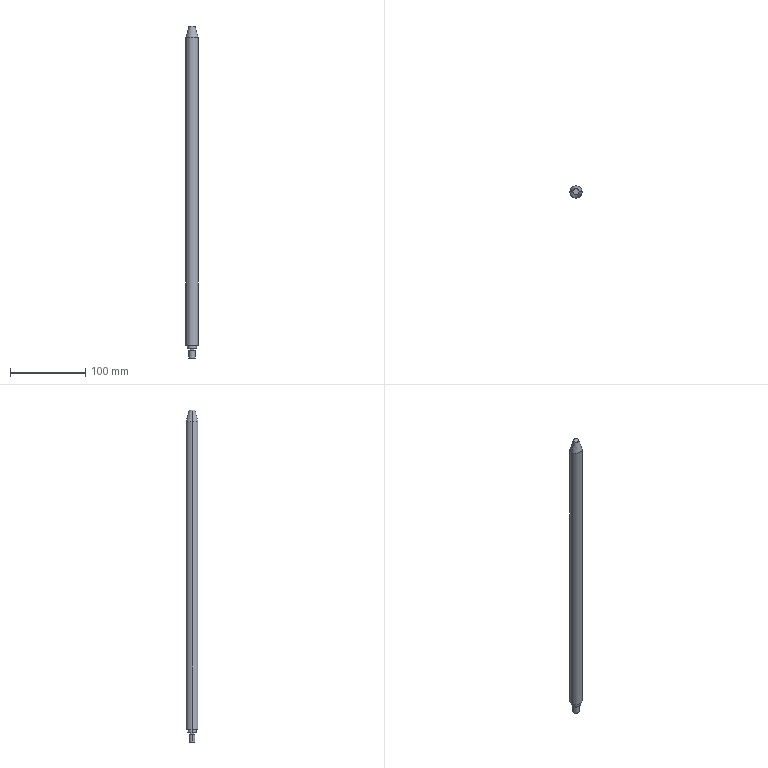Part | STEP file | Stop rod_default<machined> | 1 solid | 15 faces | box 16 x 16 x 440 mm | volume 84922 mm3 | cylinder 8 | plane 5 | cone 2 | commonest cylinder face diameters 6.5 x2 8 x2 12 x2 16 x2
STEP:
#1=CARTESIAN_POINT('',(0.,0.,0.));
#2=DIRECTION('',(0.,0.,1.));
#3=DIRECTION('',(1.,0.,0.));
#4=AXIS2_PLACEMENT_3D('',#1,#2,#3);
#5=CARTESIAN_POINT('',(6.,0.,12.));
#6=VERTEX_POINT('',#5);
#7=CARTESIAN_POINT('',(-6.,0.,12.));
#8=VERTEX_POINT('',#7);
#9=CARTESIAN_POINT('',(0.,0.,12.));
#10=DIRECTION('',(0.,0.,1.));
#11=DIRECTION('',(1.,0.,0.));
#12=AXIS2_PLACEMENT_3D('',#9,#10,#11);
#13=CIRCLE('',#12,6.);
#14=CARTESIAN_POINT('',(0.,0.,1000.));
#15=DIRECTION('',(0.,0.,1.));
#16=DIRECTION('',(1.,0.,0.));
#17=AXIS2_PLACEMENT_3D('',#14,#15,#16);
#18=CYLINDRICAL_SURFACE('',#17,6.);
#19=CARTESIAN_POINT('',(0.,-988.));
#20=DIRECTION('',(1.,0.));
#21=VECTOR('',#20,1.);
#22=LINE('',#19,#21);
#23=(GEOMETRIC_REPRESENTATION_CONTEXT(2)PARAMETRIC_REPRESENTATION_CONTEXT()REPRESENTATION_CONTEXT('',''));
#24=DEFINITIONAL_REPRESENTATION('',(#22),#23);
#25=PCURVE('',#18,#24);
#26=CARTESIAN_POINT('',(3.25,0.,12.));
#27=DIRECTION('',(0.,0.,1.));
#28=DIRECTION('',(1.,0.,0.));
#29=AXIS2_PLACEMENT_3D('',#26,#27,#28);
#30=PLANE('',#29);
#31=CARTESIAN_POINT('',(-3.25,0.));
#32=DIRECTION('',(1.,0.));
#33=AXIS2_PLACEMENT_2D('',#31,#32);
#34=CIRCLE('',#33,6.);
#35=(GEOMETRIC_REPRESENTATION_CONTEXT(2)PARAMETRIC_REPRESENTATION_CONTEXT()REPRESENTATION_CONTEXT('',''));
#36=DEFINITIONAL_REPRESENTATION('',(#34),#35);
#37=PCURVE('',#30,#36);
#38=SURFACE_CURVE('',#13,(#25,#37),.PCURVE_S1.);
#39=EDGE_CURVE('',#6,#8,#38,.T.);
#40=ORIENTED_EDGE('',*,*,#39,.T.);
#41=CARTESIAN_POINT('',(-6.,0.,17.));
#42=VERTEX_POINT('',#41);
#43=CARTESIAN_POINT('',(-6.,0.,1000.));
#44=DIRECTION('',(0.,0.,1.));
#45=VECTOR('',#44,1.);
#46=LINE('',#43,#45);
#47=CARTESIAN_POINT('',(3.142,0.));
#48=DIRECTION('',(0.,1.));
#49=VECTOR('',#48,1.);
#50=LINE('',#47,#49);
#51=(GEOMETRIC_REPRESENTATION_CONTEXT(2)PARAMETRIC_REPRESENTATION_CONTEXT()REPRESENTATION_CONTEXT('',''));
#52=DEFINITIONAL_REPRESENTATION('',(#50),#51);
#53=PCURVE('',#18,#52);
#54=CARTESIAN_POINT('',(0.,0.,1000.));
#55=DIRECTION('',(0.,0.,1.));
#56=DIRECTION('',(1.,0.,0.));
#57=AXIS2_PLACEMENT_3D('',#54,#55,#56);
#58=CYLINDRICAL_SURFACE('',#57,6.);
#59=CARTESIAN_POINT('',(3.142,0.));
#60=DIRECTION('',(0.,1.));
#61=VECTOR('',#60,1.);
#62=LINE('',#59,#61);
#63=(GEOMETRIC_REPRESENTATION_CONTEXT(2)PARAMETRIC_REPRESENTATION_CONTEXT()REPRESENTATION_CONTEXT('',''));
#64=DEFINITIONAL_REPRESENTATION('',(#62),#63);
#65=PCURVE('',#58,#64);
#66=SURFACE_CURVE('',#46,(#53,#65),.PCURVE_S1.);
#67=EDGE_CURVE('',#8,#42,#66,.T.);
#68=ORIENTED_EDGE('',*,*,#67,.T.);
#69=CARTESIAN_POINT('',(6.,0.,17.));
#70=VERTEX_POINT('',#69);
#71=CARTESIAN_POINT('',(0.,0.,17.));
#72=DIRECTION('',(0.,0.,1.));
#73=DIRECTION('',(1.,0.,0.));
#74=AXIS2_PLACEMENT_3D('',#71,#72,#73);
#75=CIRCLE('',#74,6.);
#76=CARTESIAN_POINT('',(0.,-983.));
#77=DIRECTION('',(1.,0.));
#78=VECTOR('',#77,1.);
#79=LINE('',#76,#78);
#80=(GEOMETRIC_REPRESENTATION_CONTEXT(2)PARAMETRIC_REPRESENTATION_CONTEXT()REPRESENTATION_CONTEXT('',''));
#81=DEFINITIONAL_REPRESENTATION('',(#79),#80);
#82=PCURVE('',#18,#81);
#83=CARTESIAN_POINT('',(6.,0.,17.));
#84=DIRECTION('',(0.,0.,1.));
#85=DIRECTION('',(1.,0.,0.));
#86=AXIS2_PLACEMENT_3D('',#83,#84,#85);
#87=PLANE('',#86);
#88=CARTESIAN_POINT('',(-6.,0.));
#89=DIRECTION('',(1.,0.));
#90=AXIS2_PLACEMENT_2D('',#88,#89);
#91=CIRCLE('',#90,6.);
#92=(GEOMETRIC_REPRESENTATION_CONTEXT(2)PARAMETRIC_REPRESENTATION_CONTEXT()REPRESENTATION_CONTEXT('',''));
#93=DEFINITIONAL_REPRESENTATION('',(#91),#92);
#94=PCURVE('',#87,#93);
#95=SURFACE_CURVE('',#75,(#82,#94),.PCURVE_S1.);
#96=EDGE_CURVE('',#70,#42,#95,.T.);
#97=ORIENTED_EDGE('',*,*,#96,.F.);
#98=CARTESIAN_POINT('',(6.,0.,1000.));
#99=DIRECTION('',(0.,0.,1.));
#100=VECTOR('',#99,1.);
#101=LINE('',#98,#100);
#102=CARTESIAN_POINT('',(0.,0.));
#103=DIRECTION('',(0.,1.));
#104=VECTOR('',#103,1.);
#105=LINE('',#102,#104);
#106=(GEOMETRIC_REPRESENTATION_CONTEXT(2)PARAMETRIC_REPRESENTATION_CONTEXT()REPRESENTATION_CONTEXT('',''));
#107=DEFINITIONAL_REPRESENTATION('',(#105),#106);
#108=PCURVE('',#18,#107);
#109=CARTESIAN_POINT('',(6.283,0.));
#110=DIRECTION('',(0.,1.));
#111=VECTOR('',#110,1.);
#112=LINE('',#109,#111);
#113=(GEOMETRIC_REPRESENTATION_CONTEXT(2)PARAMETRIC_REPRESENTATION_CONTEXT()REPRESENTATION_CONTEXT('',''));
#114=DEFINITIONAL_REPRESENTATION('',(#112),#113);
#115=PCURVE('',#58,#114);
#116=SURFACE_CURVE('',#101,(#108,#115),.PCURVE_S1.);
#117=EDGE_CURVE('',#6,#70,#116,.T.);
#118=ORIENTED_EDGE('',*,*,#117,.F.);
#119=EDGE_LOOP('',(#40,#68,#97,#118));
#120=FACE_BOUND('',#119,.T.);
#121=ADVANCED_FACE('',(#120),#18,.T.);
#122=CARTESIAN_POINT('',(3.25,0.,10.));
#123=VERTEX_POINT('',#122);
#124=CARTESIAN_POINT('',(-3.25,0.,10.));
#125=VERTEX_POINT('',#124);
#126=CARTESIAN_POINT('',(0.,0.,10.));
#127=DIRECTION('',(0.,0.,1.));
#128=DIRECTION('',(1.,0.,0.));
#129=AXIS2_PLACEMENT_3D('',#126,#127,#128);
#130=CIRCLE('',#129,3.25);
#131=CARTESIAN_POINT('',(0.,0.,1000.));
#132=DIRECTION('',(0.,0.,1.));
#133=DIRECTION('',(1.,0.,0.));
#134=AXIS2_PLACEMENT_3D('',#131,#132,#133);
#135=CYLINDRICAL_SURFACE('',#134,3.25);
#136=CARTESIAN_POINT('',(0.,-990.));
#137=DIRECTION('',(1.,0.));
#138=VECTOR('',#137,1.);
#139=LINE('',#136,#138);
#140=(GEOMETRIC_REPRESENTATION_CONTEXT(2)PARAMETRIC_REPRESENTATION_CONTEXT()REPRESENTATION_CONTEXT('',''));
#141=DEFINITIONAL_REPRESENTATION('',(#139),#140);
#142=PCURVE('',#135,#141);
#143=CARTESIAN_POINT('',(4.,0.,10.));
#144=DIRECTION('',(0.,0.,-1.));
#145=DIRECTION('',(-1.,0.,0.));
#146=AXIS2_PLACEMENT_3D('',#143,#144,#145);
#147=PLANE('',#146);
#148=CARTESIAN_POINT('',(0.75,0.));
#149=CARTESIAN_POINT('',(0.75,5.629));
#150=CARTESIAN_POINT('',(5.625,2.815));
#151=CARTESIAN_POINT('',(10.5,0.));
#152=CARTESIAN_POINT('',(5.625,-2.815));
#153=CARTESIAN_POINT('',(0.75,-5.629));
#154=CARTESIAN_POINT('',(0.75,0.));
#155=(BOUNDED_CURVE()B_SPLINE_CURVE(2,(#148,#149,#150,#151,#152,#153,#154),.UNSPECIFIED.,.T.,.F.)B_SPLINE_CURVE_WITH_KNOTS((1,2,2,2,2,1),(-2.094,0.,2.094,4.189,6.283,8.378),.UNSPECIFIED.)CURVE()GEOMETRIC_REPRESENTATION_ITEM()RATIONAL_B_SPLINE_CURVE((1.,0.5,1.,0.5,1.,0.5,1.))REPRESENTATION_ITEM(''));
#156=(GEOMETRIC_REPRESENTATION_CONTEXT(2)PARAMETRIC_REPRESENTATION_CONTEXT()REPRESENTATION_CONTEXT('',''));
#157=DEFINITIONAL_REPRESENTATION('',(#155),#156);
#158=PCURVE('',#147,#157);
#159=SURFACE_CURVE('',#130,(#142,#158),.PCURVE_S1.);
#160=EDGE_CURVE('',#123,#125,#159,.T.);
#161=ORIENTED_EDGE('',*,*,#160,.T.);
#162=CARTESIAN_POINT('',(-3.25,0.,12.));
#163=VERTEX_POINT('',#162);
#164=CARTESIAN_POINT('',(-3.25,0.,1000.));
#165=DIRECTION('',(0.,0.,1.));
#166=VECTOR('',#165,1.);
#167=LINE('',#164,#166);
#168=CARTESIAN_POINT('',(3.142,0.));
#169=DIRECTION('',(0.,1.));
#170=VECTOR('',#169,1.);
#171=LINE('',#168,#170);
#172=(GEOMETRIC_REPRESENTATION_CONTEXT(2)PARAMETRIC_REPRESENTATION_CONTEXT()REPRESENTATION_CONTEXT('',''));
#173=DEFINITIONAL_REPRESENTATION('',(#171),#172);
#174=PCURVE('',#135,#173);
#175=CARTESIAN_POINT('',(0.,0.,1000.));
#176=DIRECTION('',(0.,0.,1.));
#177=DIRECTION('',(1.,0.,0.));
#178=AXIS2_PLACEMENT_3D('',#175,#176,#177);
#179=CYLINDRICAL_SURFACE('',#178,3.25);
#180=CARTESIAN_POINT('',(3.142,0.));
#181=DIRECTION('',(0.,1.));
#182=VECTOR('',#181,1.);
#183=LINE('',#180,#182);
#184=(GEOMETRIC_REPRESENTATION_CONTEXT(2)PARAMETRIC_REPRESENTATION_CONTEXT()REPRESENTATION_CONTEXT('',''));
#185=DEFINITIONAL_REPRESENTATION('',(#183),#184);
#186=PCURVE('',#179,#185);
#187=SURFACE_CURVE('',#167,(#174,#186),.PCURVE_S1.);
#188=EDGE_CURVE('',#125,#163,#187,.T.);
#189=ORIENTED_EDGE('',*,*,#188,.T.);
#190=CARTESIAN_POINT('',(3.25,0.,12.));
#191=VERTEX_POINT('',#190);
#192=CARTESIAN_POINT('',(0.,0.,12.));
#193=DIRECTION('',(0.,0.,1.));
#194=DIRECTION('',(1.,0.,0.));
#195=AXIS2_PLACEMENT_3D('',#192,#193,#194);
#196=CIRCLE('',#195,3.25);
#197=CARTESIAN_POINT('',(0.,-988.));
#198=DIRECTION('',(1.,0.));
#199=VECTOR('',#198,1.);
#200=LINE('',#197,#199);
#201=(GEOMETRIC_REPRESENTATION_CONTEXT(2)PARAMETRIC_REPRESENTATION_CONTEXT()REPRESENTATION_CONTEXT('',''));
#202=DEFINITIONAL_REPRESENTATION('',(#200),#201);
#203=PCURVE('',#135,#202);
#204=CARTESIAN_POINT('',(-3.25,0.));
#205=DIRECTION('',(1.,0.));
#206=AXIS2_PLACEMENT_2D('',#204,#205);
#207=CIRCLE('',#206,3.25);
#208=(GEOMETRIC_REPRESENTATION_CONTEXT(2)PARAMETRIC_REPRESENTATION_CONTEXT()REPRESENTATION_CONTEXT('',''));
#209=DEFINITIONAL_REPRESENTATION('',(#207),#208);
#210=PCURVE('',#30,#209);
#211=SURFACE_CURVE('',#196,(#203,#210),.PCURVE_S1.);
#212=EDGE_CURVE('',#191,#163,#211,.T.);
#213=ORIENTED_EDGE('',*,*,#212,.F.);
#214=CARTESIAN_POINT('',(3.25,0.,1000.));
#215=DIRECTION('',(0.,0.,1.));
#216=VECTOR('',#215,1.);
#217=LINE('',#214,#216);
#218=CARTESIAN_POINT('',(0.,0.));
#219=DIRECTION('',(0.,1.));
#220=VECTOR('',#219,1.);
#221=LINE('',#218,#220);
#222=(GEOMETRIC_REPRESENTATION_CONTEXT(2)PARAMETRIC_REPRESENTATION_CONTEXT()REPRESENTATION_CONTEXT('',''));
#223=DEFINITIONAL_REPRESENTATION('',(#221),#222);
#224=PCURVE('',#135,#223);
#225=CARTESIAN_POINT('',(6.283,0.));
#226=DIRECTION('',(0.,1.));
#227=VECTOR('',#226,1.);
#228=LINE('',#225,#227);
#229=(GEOMETRIC_REPRESENTATION_CONTEXT(2)PARAMETRIC_REPRESENTATION_CONTEXT()REPRESENTATION_CONTEXT('',''));
#230=DEFINITIONAL_REPRESENTATION('',(#228),#229);
#231=PCURVE('',#179,#230);
#232=SURFACE_CURVE('',#217,(#224,#231),.PCURVE_S1.);
#233=EDGE_CURVE('',#123,#191,#232,.T.);
#234=ORIENTED_EDGE('',*,*,#233,.F.);
#235=EDGE_LOOP('',(#161,#189,#213,#234));
#236=FACE_BOUND('',#235,.T.);
#237=ADVANCED_FACE('',(#236),#135,.T.);
#238=CARTESIAN_POINT('',(4.,0.,0.));
#239=VERTEX_POINT('',#238);
#240=CARTESIAN_POINT('',(-4.,0.,0.));
#241=VERTEX_POINT('',#240);
#242=CARTESIAN_POINT('',(0.,0.,0.));
#243=DIRECTION('',(0.,0.,1.));
#244=DIRECTION('',(1.,0.,0.));
#245=AXIS2_PLACEMENT_3D('',#242,#243,#244);
#246=CIRCLE('',#245,4.);
#247=CARTESIAN_POINT('',(0.,0.,1000.));
#248=DIRECTION('',(0.,0.,1.));
#249=DIRECTION('',(1.,0.,0.));
#250=AXIS2_PLACEMENT_3D('',#247,#248,#249);
#251=CYLINDRICAL_SURFACE('',#250,4.);
#252=CARTESIAN_POINT('',(0.,-1000.));
#253=DIRECTION('',(1.,0.));
#254=VECTOR('',#253,1.);
#255=LINE('',#252,#254);
#256=(GEOMETRIC_REPRESENTATION_CONTEXT(2)PARAMETRIC_REPRESENTATION_CONTEXT()REPRESENTATION_CONTEXT('',''));
#257=DEFINITIONAL_REPRESENTATION('',(#255),#256);
#258=PCURVE('',#251,#257);
#259=CARTESIAN_POINT('',(0.,0.,0.));
#260=DIRECTION('',(0.,0.,1.));
#261=DIRECTION('',(1.,0.,0.));
#262=AXIS2_PLACEMENT_3D('',#259,#260,#261);
#263=PLANE('',#262);
#264=CARTESIAN_POINT('',(0.,0.));
#265=DIRECTION('',(1.,0.));
#266=AXIS2_PLACEMENT_2D('',#264,#265);
#267=CIRCLE('',#266,4.);
#268=(GEOMETRIC_REPRESENTATION_CONTEXT(2)PARAMETRIC_REPRESENTATION_CONTEXT()REPRESENTATION_CONTEXT('',''));
#269=DEFINITIONAL_REPRESENTATION('',(#267),#268);
#270=PCURVE('',#263,#269);
#271=SURFACE_CURVE('',#246,(#258,#270),.PCURVE_S1.);
#272=EDGE_CURVE('',#239,#241,#271,.T.);
#273=ORIENTED_EDGE('',*,*,#272,.T.);
#274=CARTESIAN_POINT('',(-4.,0.,10.));
#275=VERTEX_POINT('',#274);
#276=CARTESIAN_POINT('',(-4.,0.,1000.));
#277=DIRECTION('',(0.,0.,1.));
#278=VECTOR('',#277,1.);
#279=LINE('',#276,#278);
#280=CARTESIAN_POINT('',(3.142,0.));
#281=DIRECTION('',(0.,1.));
#282=VECTOR('',#281,1.);
#283=LINE('',#280,#282);
#284=(GEOMETRIC_REPRESENTATION_CONTEXT(2)PARAMETRIC_REPRESENTATION_CONTEXT()REPRESENTATION_CONTEXT('',''));
#285=DEFINITIONAL_REPRESENTATION('',(#283),#284);
#286=PCURVE('',#251,#285);
#287=CARTESIAN_POINT('',(0.,0.,1000.));
#288=DIRECTION('',(0.,0.,1.));
#289=DIRECTION('',(1.,0.,0.));
#290=AXIS2_PLACEMENT_3D('',#287,#288,#289);
#291=CYLINDRICAL_SURFACE('',#290,4.);
#292=CARTESIAN_POINT('',(3.142,0.));
#293=DIRECTION('',(0.,1.));
#294=VECTOR('',#293,1.);
#295=LINE('',#292,#294);
#296=(GEOMETRIC_REPRESENTATION_CONTEXT(2)PARAMETRIC_REPRESENTATION_CONTEXT()REPRESENTATION_CONTEXT('',''));
#297=DEFINITIONAL_REPRESENTATION('',(#295),#296);
#298=PCURVE('',#291,#297);
#299=SURFACE_CURVE('',#279,(#286,#298),.PCURVE_S1.);
#300=EDGE_CURVE('',#241,#275,#299,.T.);
#301=ORIENTED_EDGE('',*,*,#300,.T.);
#302=CARTESIAN_POINT('',(4.,0.,10.));
#303=VERTEX_POINT('',#302);
#304=CARTESIAN_POINT('',(0.,0.,10.));
#305=DIRECTION('',(0.,0.,1.));
#306=DIRECTION('',(1.,0.,0.));
#307=AXIS2_PLACEMENT_3D('',#304,#305,#306);
#308=CIRCLE('',#307,4.);
#309=CARTESIAN_POINT('',(0.,-990.));
#310=DIRECTION('',(1.,0.));
#311=VECTOR('',#310,1.);
#312=LINE('',#309,#311);
#313=(GEOMETRIC_REPRESENTATION_CONTEXT(2)PARAMETRIC_REPRESENTATION_CONTEXT()REPRESENTATION_CONTEXT('',''));
#314=DEFINITIONAL_REPRESENTATION('',(#312),#313);
#315=PCURVE('',#251,#314);
#316=CARTESIAN_POINT('',(0.,0.));
#317=CARTESIAN_POINT('',(0.,6.928));
#318=CARTESIAN_POINT('',(6.,3.464));
#319=CARTESIAN_POINT('',(12.,0.));
#320=CARTESIAN_POINT('',(6.,-3.464));
#321=CARTESIAN_POINT('',(0.,-6.928));
#322=CARTESIAN_POINT('',(0.,0.));
#323=(BOUNDED_CURVE()B_SPLINE_CURVE(2,(#316,#317,#318,#319,#320,#321,#322),.UNSPECIFIED.,.T.,.F.)B_SPLINE_CURVE_WITH_KNOTS((1,2,2,2,2,1),(-2.094,0.,2.094,4.189,6.283,8.378),.UNSPECIFIED.)CURVE()GEOMETRIC_REPRESENTATION_ITEM()RATIONAL_B_SPLINE_CURVE((1.,0.5,1.,0.5,1.,0.5,1.))REPRESENTATION_ITEM(''));
#324=(GEOMETRIC_REPRESENTATION_CONTEXT(2)PARAMETRIC_REPRESENTATION_CONTEXT()REPRESENTATION_CONTEXT('',''));
#325=DEFINITIONAL_REPRESENTATION('',(#323),#324);
#326=PCURVE('',#147,#325);
#327=SURFACE_CURVE('',#308,(#315,#326),.PCURVE_S1.);
#328=EDGE_CURVE('',#303,#275,#327,.T.);
#329=ORIENTED_EDGE('',*,*,#328,.F.);
#330=CARTESIAN_POINT('',(4.,0.,1000.));
#331=DIRECTION('',(0.,0.,1.));
#332=VECTOR('',#331,1.);
#333=LINE('',#330,#332);
#334=CARTESIAN_POINT('',(0.,0.));
#335=DIRECTION('',(0.,1.));
#336=VECTOR('',#335,1.);
#337=LINE('',#334,#336);
#338=(GEOMETRIC_REPRESENTATION_CONTEXT(2)PARAMETRIC_REPRESENTATION_CONTEXT()REPRESENTATION_CONTEXT('',''));
#339=DEFINITIONAL_REPRESENTATION('',(#337),#338);
#340=PCURVE('',#251,#339);
#341=CARTESIAN_POINT('',(6.283,0.));
#342=DIRECTION('',(0.,1.));
#343=VECTOR('',#342,1.);
#344=LINE('',#341,#343);
#345=(GEOMETRIC_REPRESENTATION_CONTEXT(2)PARAMETRIC_REPRESENTATION_CONTEXT()REPRESENTATION_CONTEXT('',''));
#346=DEFINITIONAL_REPRESENTATION('',(#344),#345);
#347=PCURVE('',#291,#346);
#348=SURFACE_CURVE('',#333,(#340,#347),.PCURVE_S1.);
#349=EDGE_CURVE('',#239,#303,#348,.T.);
#350=ORIENTED_EDGE('',*,*,#349,.F.);
#351=EDGE_LOOP('',(#273,#301,#329,#350));
#352=FACE_BOUND('',#351,.T.);
#353=ADVANCED_FACE('',(#352),#251,.T.);
#354=CARTESIAN_POINT('',(3.981,0.,440.));
#355=VERTEX_POINT('',#354);
#356=CARTESIAN_POINT('',(-3.981,0.,440.));
#357=VERTEX_POINT('',#356);
#358=CARTESIAN_POINT('',(0.,0.,440.));
#359=DIRECTION('',(0.,0.,1.));
#360=DIRECTION('',(1.,0.,0.));
#361=AXIS2_PLACEMENT_3D('',#358,#359,#360);
#362=CIRCLE('',#361,3.981);
#363=CARTESIAN_POINT('',(0.,0.,440.));
#364=DIRECTION('',(0.,0.,-1.));
#365=DIRECTION('',(-1.,0.,0.));
#366=AXIS2_PLACEMENT_3D('',#363,#364,#365);
#367=CONICAL_SURFACE('',#366,3.981,0.2618);
#368=CARTESIAN_POINT('',(3.142,0.));
#369=DIRECTION('',(-1.,0.));
#370=VECTOR('',#369,1.);
#371=LINE('',#368,#370);
#372=(GEOMETRIC_REPRESENTATION_CONTEXT(2)PARAMETRIC_REPRESENTATION_CONTEXT()REPRESENTATION_CONTEXT('',''));
#373=DEFINITIONAL_REPRESENTATION('',(#371),#372);
#374=PCURVE('',#367,#373);
#375=CARTESIAN_POINT('',(0.,0.,440.));
#376=DIRECTION('',(0.,0.,1.));
#377=DIRECTION('',(1.,0.,0.));
#378=AXIS2_PLACEMENT_3D('',#375,#376,#377);
#379=PLANE('',#378);
#380=CARTESIAN_POINT('',(0.,0.));
#381=DIRECTION('',(1.,0.));
#382=AXIS2_PLACEMENT_2D('',#380,#381);
#383=CIRCLE('',#382,3.981);
#384=(GEOMETRIC_REPRESENTATION_CONTEXT(2)PARAMETRIC_REPRESENTATION_CONTEXT()REPRESENTATION_CONTEXT('',''));
#385=DEFINITIONAL_REPRESENTATION('',(#383),#384);
#386=PCURVE('',#379,#385);
#387=SURFACE_CURVE('',#362,(#374,#386),.PCURVE_S1.);
#388=EDGE_CURVE('',#355,#357,#387,.T.);
#389=ORIENTED_EDGE('',*,*,#388,.F.);
#390=CARTESIAN_POINT('',(8.,0.,425.));
#391=VERTEX_POINT('',#390);
#392=CARTESIAN_POINT('',(3.981,0.,440.));
#393=DIRECTION('',(0.2588,0.,-0.9659));
#394=VECTOR('',#393,1.);
#395=LINE('',#392,#394);
#396=CARTESIAN_POINT('',(3.142,0.));
#397=DIRECTION('',(0.,1.));
#398=VECTOR('',#397,1.);
#399=LINE('',#396,#398);
#400=(GEOMETRIC_REPRESENTATION_CONTEXT(2)PARAMETRIC_REPRESENTATION_CONTEXT()REPRESENTATION_CONTEXT('',''));
#401=DEFINITIONAL_REPRESENTATION('',(#399),#400);
#402=PCURVE('',#367,#401);
#403=CARTESIAN_POINT('',(0.,0.,440.));
#404=DIRECTION('',(0.,0.,-1.));
#405=DIRECTION('',(-1.,0.,0.));
#406=AXIS2_PLACEMENT_3D('',#403,#404,#405);
#407=CONICAL_SURFACE('',#406,3.981,0.2618);
#408=CARTESIAN_POINT('',(3.142,0.));
#409=DIRECTION('',(0.,1.));
#410=VECTOR('',#409,1.);
#411=LINE('',#408,#410);
#412=(GEOMETRIC_REPRESENTATION_CONTEXT(2)PARAMETRIC_REPRESENTATION_CONTEXT()REPRESENTATION_CONTEXT('',''));
#413=DEFINITIONAL_REPRESENTATION('',(#411),#412);
#414=PCURVE('',#407,#413);
#415=SURFACE_CURVE('',#395,(#402,#414),.PCURVE_S1.);
#416=EDGE_CURVE('',#355,#391,#415,.T.);
#417=ORIENTED_EDGE('',*,*,#416,.T.);
#418=CARTESIAN_POINT('',(-8.,0.,425.));
#419=VERTEX_POINT('',#418);
#420=CARTESIAN_POINT('',(0.,0.,425.));
#421=DIRECTION('',(0.,0.,-1.));
#422=DIRECTION('',(1.,0.,0.));
#423=AXIS2_PLACEMENT_3D('',#420,#421,#422);
#424=CIRCLE('',#423,8.);
#425=CARTESIAN_POINT('',(-3.142,15.));
#426=DIRECTION('',(1.,0.));
#427=VECTOR('',#426,1.);
#428=LINE('',#425,#427);
#429=(GEOMETRIC_REPRESENTATION_CONTEXT(2)PARAMETRIC_REPRESENTATION_CONTEXT()REPRESENTATION_CONTEXT('',''));
#430=DEFINITIONAL_REPRESENTATION('',(#428),#429);
#431=PCURVE('',#367,#430);
#432=CARTESIAN_POINT('',(0.,0.,440.));
#433=DIRECTION('',(0.,0.,-1.));
#434=DIRECTION('',(-1.,0.,0.));
#435=AXIS2_PLACEMENT_3D('',#432,#433,#434);
#436=CYLINDRICAL_SURFACE('',#435,8.);
#437=CARTESIAN_POINT('',(-3.142,15.));
#438=DIRECTION('',(1.,0.));
#439=VECTOR('',#438,1.);
#440=LINE('',#437,#439);
#441=(GEOMETRIC_REPRESENTATION_CONTEXT(2)PARAMETRIC_REPRESENTATION_CONTEXT()REPRESENTATION_CONTEXT('',''));
#442=DEFINITIONAL_REPRESENTATION('',(#440),#441);
#443=PCURVE('',#436,#442);
#444=SURFACE_CURVE('',#424,(#431,#443),.PCURVE_S1.);
#445=EDGE_CURVE('',#419,#391,#444,.T.);
#446=ORIENTED_EDGE('',*,*,#445,.F.);
#447=CARTESIAN_POINT('',(-3.981,0.,440.));
#448=DIRECTION('',(-0.2588,0.,-0.9659));
#449=VECTOR('',#448,1.);
#450=LINE('',#447,#449);
#451=CARTESIAN_POINT('',(0.,0.));
#452=DIRECTION('',(0.,1.));
#453=VECTOR('',#452,1.);
#454=LINE('',#451,#453);
#455=(GEOMETRIC_REPRESENTATION_CONTEXT(2)PARAMETRIC_REPRESENTATION_CONTEXT()REPRESENTATION_CONTEXT('',''));
#456=DEFINITIONAL_REPRESENTATION('',(#454),#455);
#457=PCURVE('',#367,#456);
#458=CARTESIAN_POINT('',(6.283,0.));
#459=DIRECTION('',(0.,1.));
#460=VECTOR('',#459,1.);
#461=LINE('',#458,#460);
#462=(GEOMETRIC_REPRESENTATION_CONTEXT(2)PARAMETRIC_REPRESENTATION_CONTEXT()REPRESENTATION_CONTEXT('',''));
#463=DEFINITIONAL_REPRESENTATION('',(#461),#462);
#464=PCURVE('',#407,#463);
#465=SURFACE_CURVE('',#450,(#457,#464),.PCURVE_S1.);
#466=EDGE_CURVE('',#357,#419,#465,.T.);
#467=ORIENTED_EDGE('',*,*,#466,.F.);
#468=EDGE_LOOP('',(#389,#417,#446,#467));
#469=FACE_BOUND('',#468,.T.);
#470=ADVANCED_FACE('',(#469),#367,.T.);
#471=ORIENTED_EDGE('',*,*,#445,.T.);
#472=CARTESIAN_POINT('',(8.,0.,17.));
#473=VERTEX_POINT('',#472);
#474=CARTESIAN_POINT('',(8.,0.,440.));
#475=DIRECTION('',(0.,0.,-1.));
#476=VECTOR('',#475,1.);
#477=LINE('',#474,#476);
#478=CARTESIAN_POINT('',(3.142,0.));
#479=DIRECTION('',(0.,1.));
#480=VECTOR('',#479,1.);
#481=LINE('',#478,#480);
#482=(GEOMETRIC_REPRESENTATION_CONTEXT(2)PARAMETRIC_REPRESENTATION_CONTEXT()REPRESENTATION_CONTEXT('',''));
#483=DEFINITIONAL_REPRESENTATION('',(#481),#482);
#484=PCURVE('',#436,#483);
#485=CARTESIAN_POINT('',(0.,0.,440.));
#486=DIRECTION('',(0.,0.,-1.));
#487=DIRECTION('',(-1.,0.,0.));
#488=AXIS2_PLACEMENT_3D('',#485,#486,#487);
#489=CYLINDRICAL_SURFACE('',#488,8.);
#490=CARTESIAN_POINT('',(3.142,0.));
#491=DIRECTION('',(0.,1.));
#492=VECTOR('',#491,1.);
#493=LINE('',#490,#492);
#494=(GEOMETRIC_REPRESENTATION_CONTEXT(2)PARAMETRIC_REPRESENTATION_CONTEXT()REPRESENTATION_CONTEXT('',''));
#495=DEFINITIONAL_REPRESENTATION('',(#493),#494);
#496=PCURVE('',#489,#495);
#497=SURFACE_CURVE('',#477,(#484,#496),.PCURVE_S1.);
#498=EDGE_CURVE('',#391,#473,#497,.T.);
#499=ORIENTED_EDGE('',*,*,#498,.T.);
#500=CARTESIAN_POINT('',(-8.,0.,17.));
#501=VERTEX_POINT('',#500);
#502=CARTESIAN_POINT('',(0.,0.,17.));
#503=DIRECTION('',(0.,0.,1.));
#504=DIRECTION('',(1.,0.,0.));
#505=AXIS2_PLACEMENT_3D('',#502,#503,#504);
#506=CIRCLE('',#505,8.);
#507=CARTESIAN_POINT('',(3.142,423.));
#508=DIRECTION('',(-1.,0.));
#509=VECTOR('',#508,1.);
#510=LINE('',#507,#509);
#511=(GEOMETRIC_REPRESENTATION_CONTEXT(2)PARAMETRIC_REPRESENTATION_CONTEXT()REPRESENTATION_CONTEXT('',''));
#512=DEFINITIONAL_REPRESENTATION('',(#510),#511);
#513=PCURVE('',#436,#512);
#514=CARTESIAN_POINT('',(-6.,0.));
#515=DIRECTION('',(1.,0.));
#516=AXIS2_PLACEMENT_2D('',#514,#515);
#517=CIRCLE('',#516,8.);
#518=(GEOMETRIC_REPRESENTATION_CONTEXT(2)PARAMETRIC_REPRESENTATION_CONTEXT()REPRESENTATION_CONTEXT('',''));
#519=DEFINITIONAL_REPRESENTATION('',(#517),#518);
#520=PCURVE('',#87,#519);
#521=SURFACE_CURVE('',#506,(#513,#520),.PCURVE_S1.);
#522=EDGE_CURVE('',#473,#501,#521,.T.);
#523=ORIENTED_EDGE('',*,*,#522,.T.);
#524=CARTESIAN_POINT('',(-8.,0.,440.));
#525=DIRECTION('',(0.,0.,-1.));
#526=VECTOR('',#525,1.);
#527=LINE('',#524,#526);
#528=CARTESIAN_POINT('',(0.,0.));
#529=DIRECTION('',(0.,1.));
#530=VECTOR('',#529,1.);
#531=LINE('',#528,#530);
#532=(GEOMETRIC_REPRESENTATION_CONTEXT(2)PARAMETRIC_REPRESENTATION_CONTEXT()REPRESENTATION_CONTEXT('',''));
#533=DEFINITIONAL_REPRESENTATION('',(#531),#532);
#534=PCURVE('',#436,#533);
#535=CARTESIAN_POINT('',(6.283,0.));
#536=DIRECTION('',(0.,1.));
#537=VECTOR('',#536,1.);
#538=LINE('',#535,#537);
#539=(GEOMETRIC_REPRESENTATION_CONTEXT(2)PARAMETRIC_REPRESENTATION_CONTEXT()REPRESENTATION_CONTEXT('',''));
#540=DEFINITIONAL_REPRESENTATION('',(#538),#539);
#541=PCURVE('',#489,#540);
#542=SURFACE_CURVE('',#527,(#534,#541),.PCURVE_S1.);
#543=EDGE_CURVE('',#419,#501,#542,.T.);
#544=ORIENTED_EDGE('',*,*,#543,.F.);
#545=EDGE_LOOP('',(#471,#499,#523,#544));
#546=FACE_BOUND('',#545,.T.);
#547=ADVANCED_FACE('',(#546),#436,.T.);
#548=ORIENTED_EDGE('',*,*,#498,.F.);
#549=CARTESIAN_POINT('',(0.,0.,425.));
#550=DIRECTION('',(0.,0.,-1.));
#551=DIRECTION('',(1.,0.,0.));
#552=AXIS2_PLACEMENT_3D('',#549,#550,#551);
#553=CIRCLE('',#552,8.);
#554=CARTESIAN_POINT('',(3.142,15.));
#555=DIRECTION('',(1.,0.));
#556=VECTOR('',#555,1.);
#557=LINE('',#554,#556);
#558=(GEOMETRIC_REPRESENTATION_CONTEXT(2)PARAMETRIC_REPRESENTATION_CONTEXT()REPRESENTATION_CONTEXT('',''));
#559=DEFINITIONAL_REPRESENTATION('',(#557),#558);
#560=PCURVE('',#489,#559);
#561=CARTESIAN_POINT('',(3.142,15.));
#562=DIRECTION('',(1.,0.));
#563=VECTOR('',#562,1.);
#564=LINE('',#561,#563);
#565=(GEOMETRIC_REPRESENTATION_CONTEXT(2)PARAMETRIC_REPRESENTATION_CONTEXT()REPRESENTATION_CONTEXT('',''));
#566=DEFINITIONAL_REPRESENTATION('',(#564),#565);
#567=PCURVE('',#407,#566);
#568=SURFACE_CURVE('',#553,(#560,#567),.PCURVE_S1.);
#569=EDGE_CURVE('',#391,#419,#568,.T.);
#570=ORIENTED_EDGE('',*,*,#569,.T.);
#571=ORIENTED_EDGE('',*,*,#543,.T.);
#572=CARTESIAN_POINT('',(0.,0.,17.));
#573=DIRECTION('',(0.,0.,1.));
#574=DIRECTION('',(1.,0.,0.));
#575=AXIS2_PLACEMENT_3D('',#572,#573,#574);
#576=CIRCLE('',#575,8.);
#577=CARTESIAN_POINT('',(9.425,423.));
#578=DIRECTION('',(-1.,0.));
#579=VECTOR('',#578,1.);
#580=LINE('',#577,#579);
#581=(GEOMETRIC_REPRESENTATION_CONTEXT(2)PARAMETRIC_REPRESENTATION_CONTEXT()REPRESENTATION_CONTEXT('',''));
#582=DEFINITIONAL_REPRESENTATION('',(#580),#581);
#583=PCURVE('',#489,#582);
#584=CARTESIAN_POINT('',(-6.,0.));
#585=DIRECTION('',(1.,0.));
#586=AXIS2_PLACEMENT_2D('',#584,#585);
#587=CIRCLE('',#586,8.);
#588=(GEOMETRIC_REPRESENTATION_CONTEXT(2)PARAMETRIC_REPRESENTATION_CONTEXT()REPRESENTATION_CONTEXT('',''));
#589=DEFINITIONAL_REPRESENTATION('',(#587),#588);
#590=PCURVE('',#87,#589);
#591=SURFACE_CURVE('',#576,(#583,#590),.PCURVE_S1.);
#592=EDGE_CURVE('',#501,#473,#591,.T.);
#593=ORIENTED_EDGE('',*,*,#592,.T.);
#594=EDGE_LOOP('',(#548,#570,#571,#593));
#595=FACE_BOUND('',#594,.T.);
#596=ADVANCED_FACE('',(#595),#489,.T.);
#597=CARTESIAN_POINT('',(0.,0.,440.));
#598=DIRECTION('',(0.,0.,1.));
#599=DIRECTION('',(1.,0.,0.));
#600=AXIS2_PLACEMENT_3D('',#597,#598,#599);
#601=CIRCLE('',#600,3.981);
#602=CARTESIAN_POINT('',(0.,0.));
#603=DIRECTION('',(1.,0.));
#604=AXIS2_PLACEMENT_2D('',#602,#603);
#605=CIRCLE('',#604,3.981);
#606=(GEOMETRIC_REPRESENTATION_CONTEXT(2)PARAMETRIC_REPRESENTATION_CONTEXT()REPRESENTATION_CONTEXT('',''));
#607=DEFINITIONAL_REPRESENTATION('',(#605),#606);
#608=PCURVE('',#379,#607);
#609=CARTESIAN_POINT('',(9.425,0.));
#610=DIRECTION('',(-1.,0.));
#611=VECTOR('',#610,1.);
#612=LINE('',#609,#611);
#613=(GEOMETRIC_REPRESENTATION_CONTEXT(2)PARAMETRIC_REPRESENTATION_CONTEXT()REPRESENTATION_CONTEXT('',''));
#614=DEFINITIONAL_REPRESENTATION('',(#612),#613);
#615=PCURVE('',#407,#614);
#616=SURFACE_CURVE('',#601,(#608,#615),.PCURVE_S1.);
#617=EDGE_CURVE('',#357,#355,#616,.T.);
#618=ORIENTED_EDGE('',*,*,#617,.T.);
#619=ORIENTED_EDGE('',*,*,#388,.T.);
#620=EDGE_LOOP('',(#618,#619));
#621=FACE_BOUND('',#620,.T.);
#622=ADVANCED_FACE('',(#621),#379,.T.);
#623=ORIENTED_EDGE('',*,*,#416,.F.);
#624=ORIENTED_EDGE('',*,*,#617,.F.);
#625=ORIENTED_EDGE('',*,*,#466,.T.);
#626=ORIENTED_EDGE('',*,*,#569,.F.);
#627=EDGE_LOOP('',(#623,#624,#625,#626));
#628=FACE_BOUND('',#627,.T.);
#629=ADVANCED_FACE('',(#628),#407,.T.);
#630=ORIENTED_EDGE('',*,*,#300,.F.);
#631=CARTESIAN_POINT('',(0.,0.,0.));
#632=DIRECTION('',(0.,0.,1.));
#633=DIRECTION('',(1.,0.,0.));
#634=AXIS2_PLACEMENT_3D('',#631,#632,#633);
#635=CIRCLE('',#634,4.);
#636=CARTESIAN_POINT('',(0.,-1000.));
#637=DIRECTION('',(1.,0.));
#638=VECTOR('',#637,1.);
#639=LINE('',#636,#638);
#640=(GEOMETRIC_REPRESENTATION_CONTEXT(2)PARAMETRIC_REPRESENTATION_CONTEXT()REPRESENTATION_CONTEXT('',''));
#641=DEFINITIONAL_REPRESENTATION('',(#639),#640);
#642=PCURVE('',#291,#641);
#643=CARTESIAN_POINT('',(0.,0.));
#644=DIRECTION('',(1.,0.));
#645=AXIS2_PLACEMENT_2D('',#643,#644);
#646=CIRCLE('',#645,4.);
#647=(GEOMETRIC_REPRESENTATION_CONTEXT(2)PARAMETRIC_REPRESENTATION_CONTEXT()REPRESENTATION_CONTEXT('',''));
#648=DEFINITIONAL_REPRESENTATION('',(#646),#647);
#649=PCURVE('',#263,#648);
#650=SURFACE_CURVE('',#635,(#642,#649),.PCURVE_S1.);
#651=EDGE_CURVE('',#241,#239,#650,.T.);
#652=ORIENTED_EDGE('',*,*,#651,.T.);
#653=ORIENTED_EDGE('',*,*,#349,.T.);
#654=CARTESIAN_POINT('',(0.,0.,10.));
#655=DIRECTION('',(0.,0.,1.));
#656=DIRECTION('',(1.,0.,0.));
#657=AXIS2_PLACEMENT_3D('',#654,#655,#656);
#658=CIRCLE('',#657,4.);
#659=CARTESIAN_POINT('',(0.,-990.));
#660=DIRECTION('',(1.,0.));
#661=VECTOR('',#660,1.);
#662=LINE('',#659,#661);
#663=(GEOMETRIC_REPRESENTATION_CONTEXT(2)PARAMETRIC_REPRESENTATION_CONTEXT()REPRESENTATION_CONTEXT('',''));
#664=DEFINITIONAL_REPRESENTATION('',(#662),#663);
#665=PCURVE('',#291,#664);
#666=CARTESIAN_POINT('',(0.,0.));
#667=CARTESIAN_POINT('',(0.,6.928));
#668=CARTESIAN_POINT('',(6.,3.464));
#669=CARTESIAN_POINT('',(12.,0.));
#670=CARTESIAN_POINT('',(6.,-3.464));
#671=CARTESIAN_POINT('',(0.,-6.928));
#672=CARTESIAN_POINT('',(0.,0.));
#673=(BOUNDED_CURVE()B_SPLINE_CURVE(2,(#666,#667,#668,#669,#670,#671,#672),.UNSPECIFIED.,.T.,.F.)B_SPLINE_CURVE_WITH_KNOTS((1,2,2,2,2,1),(-2.094,0.,2.094,4.189,6.283,8.378),.UNSPECIFIED.)CURVE()GEOMETRIC_REPRESENTATION_ITEM()RATIONAL_B_SPLINE_CURVE((1.,0.5,1.,0.5,1.,0.5,1.))REPRESENTATION_ITEM(''));
#674=(GEOMETRIC_REPRESENTATION_CONTEXT(2)PARAMETRIC_REPRESENTATION_CONTEXT()REPRESENTATION_CONTEXT('',''));
#675=DEFINITIONAL_REPRESENTATION('',(#673),#674);
#676=PCURVE('',#147,#675);
#677=SURFACE_CURVE('',#658,(#665,#676),.PCURVE_S1.);
#678=EDGE_CURVE('',#275,#303,#677,.T.);
#679=ORIENTED_EDGE('',*,*,#678,.F.);
#680=EDGE_LOOP('',(#630,#652,#653,#679));
#681=FACE_BOUND('',#680,.T.);
#682=ADVANCED_FACE('',(#681),#291,.T.);
#683=ORIENTED_EDGE('',*,*,#160,.F.);
#684=CARTESIAN_POINT('',(0.,0.,10.));
#685=DIRECTION('',(0.,0.,1.));
#686=DIRECTION('',(1.,0.,0.));
#687=AXIS2_PLACEMENT_3D('',#684,#685,#686);
#688=CIRCLE('',#687,3.25);
#689=CARTESIAN_POINT('',(0.75,0.));
#690=CARTESIAN_POINT('',(0.75,5.629));
#691=CARTESIAN_POINT('',(5.625,2.815));
#692=CARTESIAN_POINT('',(10.5,0.));
#693=CARTESIAN_POINT('',(5.625,-2.815));
#694=CARTESIAN_POINT('',(0.75,-5.629));
#695=CARTESIAN_POINT('',(0.75,0.));
#696=(BOUNDED_CURVE()B_SPLINE_CURVE(2,(#689,#690,#691,#692,#693,#694,#695),.UNSPECIFIED.,.T.,.F.)B_SPLINE_CURVE_WITH_KNOTS((1,2,2,2,2,1),(-2.094,0.,2.094,4.189,6.283,8.378),.UNSPECIFIED.)CURVE()GEOMETRIC_REPRESENTATION_ITEM()RATIONAL_B_SPLINE_CURVE((1.,0.5,1.,0.5,1.,0.5,1.))REPRESENTATION_ITEM(''));
#697=(GEOMETRIC_REPRESENTATION_CONTEXT(2)PARAMETRIC_REPRESENTATION_CONTEXT()REPRESENTATION_CONTEXT('',''));
#698=DEFINITIONAL_REPRESENTATION('',(#696),#697);
#699=PCURVE('',#147,#698);
#700=CARTESIAN_POINT('',(0.,-990.));
#701=DIRECTION('',(1.,0.));
#702=VECTOR('',#701,1.);
#703=LINE('',#700,#702);
#704=(GEOMETRIC_REPRESENTATION_CONTEXT(2)PARAMETRIC_REPRESENTATION_CONTEXT()REPRESENTATION_CONTEXT('',''));
#705=DEFINITIONAL_REPRESENTATION('',(#703),#704);
#706=PCURVE('',#179,#705);
#707=SURFACE_CURVE('',#688,(#699,#706),.PCURVE_S1.);
#708=EDGE_CURVE('',#125,#123,#707,.T.);
#709=ORIENTED_EDGE('',*,*,#708,.F.);
#710=EDGE_LOOP('',(#683,#709));
#711=FACE_BOUND('',#710,.T.);
#712=ORIENTED_EDGE('',*,*,#328,.T.);
#713=ORIENTED_EDGE('',*,*,#678,.T.);
#714=EDGE_LOOP('',(#712,#713));
#715=FACE_BOUND('',#714,.T.);
#716=ADVANCED_FACE('',(#711,#715),#147,.F.);
#717=ORIENTED_EDGE('',*,*,#188,.F.);
#718=ORIENTED_EDGE('',*,*,#708,.T.);
#719=ORIENTED_EDGE('',*,*,#233,.T.);
#720=CARTESIAN_POINT('',(0.,0.,12.));
#721=DIRECTION('',(0.,0.,1.));
#722=DIRECTION('',(1.,0.,0.));
#723=AXIS2_PLACEMENT_3D('',#720,#721,#722);
#724=CIRCLE('',#723,3.25);
#725=CARTESIAN_POINT('',(0.,-988.));
#726=DIRECTION('',(1.,0.));
#727=VECTOR('',#726,1.);
#728=LINE('',#725,#727);
#729=(GEOMETRIC_REPRESENTATION_CONTEXT(2)PARAMETRIC_REPRESENTATION_CONTEXT()REPRESENTATION_CONTEXT('',''));
#730=DEFINITIONAL_REPRESENTATION('',(#728),#729);
#731=PCURVE('',#179,#730);
#732=CARTESIAN_POINT('',(-3.25,0.));
#733=DIRECTION('',(1.,0.));
#734=AXIS2_PLACEMENT_2D('',#732,#733);
#735=CIRCLE('',#734,3.25);
#736=(GEOMETRIC_REPRESENTATION_CONTEXT(2)PARAMETRIC_REPRESENTATION_CONTEXT()REPRESENTATION_CONTEXT('',''));
#737=DEFINITIONAL_REPRESENTATION('',(#735),#736);
#738=PCURVE('',#30,#737);
#739=SURFACE_CURVE('',#724,(#731,#738),.PCURVE_S1.);
#740=EDGE_CURVE('',#163,#191,#739,.T.);
#741=ORIENTED_EDGE('',*,*,#740,.F.);
#742=EDGE_LOOP('',(#717,#718,#719,#741));
#743=FACE_BOUND('',#742,.T.);
#744=ADVANCED_FACE('',(#743),#179,.T.);
#745=ORIENTED_EDGE('',*,*,#39,.F.);
#746=CARTESIAN_POINT('',(0.,0.,12.));
#747=DIRECTION('',(0.,0.,1.));
#748=DIRECTION('',(1.,0.,0.));
#749=AXIS2_PLACEMENT_3D('',#746,#747,#748);
#750=CIRCLE('',#749,6.);
#751=CARTESIAN_POINT('',(-3.25,0.));
#752=DIRECTION('',(1.,0.));
#753=AXIS2_PLACEMENT_2D('',#751,#752);
#754=CIRCLE('',#753,6.);
#755=(GEOMETRIC_REPRESENTATION_CONTEXT(2)PARAMETRIC_REPRESENTATION_CONTEXT()REPRESENTATION_CONTEXT('',''));
#756=DEFINITIONAL_REPRESENTATION('',(#754),#755);
#757=PCURVE('',#30,#756);
#758=CARTESIAN_POINT('',(0.,-988.));
#759=DIRECTION('',(1.,0.));
#760=VECTOR('',#759,1.);
#761=LINE('',#758,#760);
#762=(GEOMETRIC_REPRESENTATION_CONTEXT(2)PARAMETRIC_REPRESENTATION_CONTEXT()REPRESENTATION_CONTEXT('',''));
#763=DEFINITIONAL_REPRESENTATION('',(#761),#762);
#764=PCURVE('',#58,#763);
#765=SURFACE_CURVE('',#750,(#757,#764),.PCURVE_S1.);
#766=EDGE_CURVE('',#8,#6,#765,.T.);
#767=ORIENTED_EDGE('',*,*,#766,.F.);
#768=EDGE_LOOP('',(#745,#767));
#769=FACE_BOUND('',#768,.T.);
#770=ORIENTED_EDGE('',*,*,#212,.T.);
#771=ORIENTED_EDGE('',*,*,#740,.T.);
#772=EDGE_LOOP('',(#770,#771));
#773=FACE_BOUND('',#772,.T.);
#774=ADVANCED_FACE('',(#769,#773),#30,.F.);
#775=ORIENTED_EDGE('',*,*,#67,.F.);
#776=ORIENTED_EDGE('',*,*,#766,.T.);
#777=ORIENTED_EDGE('',*,*,#117,.T.);
#778=CARTESIAN_POINT('',(0.,0.,17.));
#779=DIRECTION('',(0.,0.,1.));
#780=DIRECTION('',(1.,0.,0.));
#781=AXIS2_PLACEMENT_3D('',#778,#779,#780);
#782=CIRCLE('',#781,6.);
#783=CARTESIAN_POINT('',(0.,-983.));
#784=DIRECTION('',(1.,0.));
#785=VECTOR('',#784,1.);
#786=LINE('',#783,#785);
#787=(GEOMETRIC_REPRESENTATION_CONTEXT(2)PARAMETRIC_REPRESENTATION_CONTEXT()REPRESENTATION_CONTEXT('',''));
#788=DEFINITIONAL_REPRESENTATION('',(#786),#787);
#789=PCURVE('',#58,#788);
#790=CARTESIAN_POINT('',(-6.,0.));
#791=DIRECTION('',(1.,0.));
#792=AXIS2_PLACEMENT_2D('',#790,#791);
#793=CIRCLE('',#792,6.);
#794=(GEOMETRIC_REPRESENTATION_CONTEXT(2)PARAMETRIC_REPRESENTATION_CONTEXT()REPRESENTATION_CONTEXT('',''));
#795=DEFINITIONAL_REPRESENTATION('',(#793),#794);
#796=PCURVE('',#87,#795);
#797=SURFACE_CURVE('',#782,(#789,#796),.PCURVE_S1.);
#798=EDGE_CURVE('',#42,#70,#797,.T.);
#799=ORIENTED_EDGE('',*,*,#798,.F.);
#800=EDGE_LOOP('',(#775,#776,#777,#799));
#801=FACE_BOUND('',#800,.T.);
#802=ADVANCED_FACE('',(#801),#58,.T.);
#803=ORIENTED_EDGE('',*,*,#592,.F.);
#804=ORIENTED_EDGE('',*,*,#522,.F.);
#805=EDGE_LOOP('',(#803,#804));
#806=FACE_BOUND('',#805,.T.);
#807=ORIENTED_EDGE('',*,*,#96,.T.);
#808=ORIENTED_EDGE('',*,*,#798,.T.);
#809=EDGE_LOOP('',(#807,#808));
#810=FACE_BOUND('',#809,.T.);
#811=ADVANCED_FACE('',(#806,#810),#87,.F.);
#812=ORIENTED_EDGE('',*,*,#272,.F.);
#813=ORIENTED_EDGE('',*,*,#651,.F.);
#814=EDGE_LOOP('',(#812,#813));
#815=FACE_BOUND('',#814,.T.);
#816=ADVANCED_FACE('',(#815),#263,.F.);
#817=CLOSED_SHELL('',(#121,#237,#353,#470,#547,#596,#622,#629,#682,#716,#744,#774,#802,#811,#816));
#818=MANIFOLD_SOLID_BREP('',#817);
#819=(LENGTH_UNIT()NAMED_UNIT(*)SI_UNIT(.MILLI.,.METRE.));
#820=UNCERTAINTY_MEASURE_WITH_UNIT(LENGTH_MEASURE(0.0000001),#819,'','');
#821=(NAMED_UNIT(*)PLANE_ANGLE_UNIT()SI_UNIT($,.RADIAN.));
#822=(NAMED_UNIT(*)SI_UNIT($,.STERADIAN.)SOLID_ANGLE_UNIT());
#823=(GEOMETRIC_REPRESENTATION_CONTEXT(3)GLOBAL_UNCERTAINTY_ASSIGNED_CONTEXT((#820))GLOBAL_UNIT_ASSIGNED_CONTEXT((#819,#821,#822))REPRESENTATION_CONTEXT('',''));
#824=ADVANCED_BREP_SHAPE_REPRESENTATION('',(#4,#818),#823);